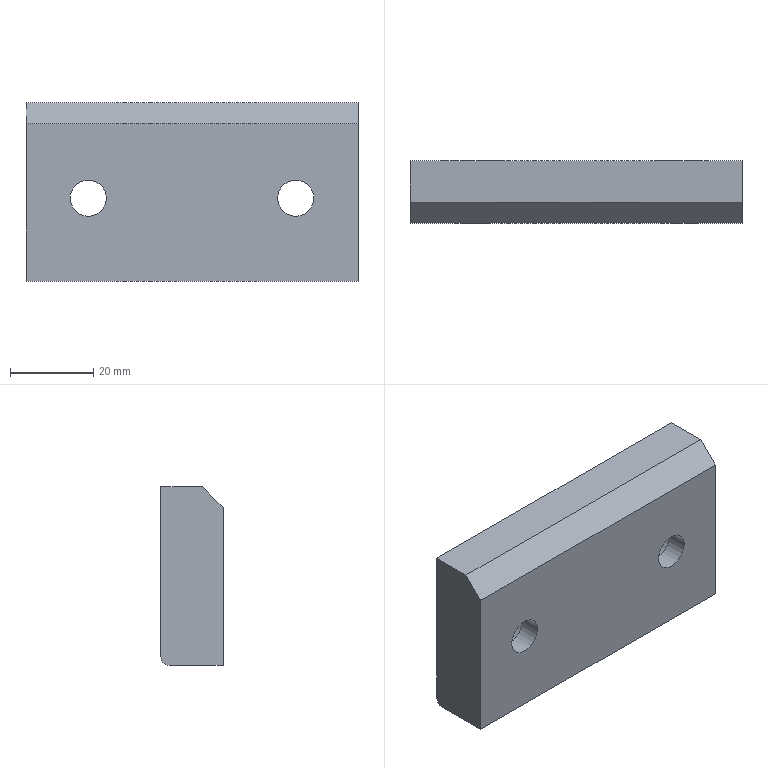Part | STEP file | 1_id1026_x_t | 1 solid | 14 faces | box 80 x 15 x 43 mm | volume 46403 mm3 | plane 9 | cylinder 5 | commonest cylinder face diameters 8.7 x2 15 x2 4 x1
STEP:
#1=CARTESIAN_POINT('',(0.,0.,0.));
#2=DIRECTION('',(0.,0.,1.));
#3=DIRECTION('',(1.,0.,0.));
#4=AXIS2_PLACEMENT_3D('',#1,#2,#3);
#5=CARTESIAN_POINT('',(787.926,422.974,-82.813));
#6=VERTEX_POINT('',#5);
#7=CARTESIAN_POINT('',(787.926,409.974,-82.813));
#8=VERTEX_POINT('',#7);
#9=CARTESIAN_POINT('',(787.926,422.974,-82.813));
#10=DIRECTION('',(0.,-1.,0.));
#11=VECTOR('',#10,1.);
#12=LINE('',#9,#11);
#13=CARTESIAN_POINT('',(787.926,409.974,-82.813));
#14=DIRECTION('',(1.,0.,0.));
#15=DIRECTION('',(0.,1.,0.));
#16=AXIS2_PLACEMENT_3D('',#13,#14,#15);
#17=PLANE('',#16);
#18=CARTESIAN_POINT('',(13.,0.));
#19=DIRECTION('',(-1.,0.));
#20=VECTOR('',#19,1.);
#21=LINE('',#18,#20);
#22=(GEOMETRIC_REPRESENTATION_CONTEXT(2)PARAMETRIC_REPRESENTATION_CONTEXT()REPRESENTATION_CONTEXT('',''));
#23=DEFINITIONAL_REPRESENTATION('',(#21),#22);
#24=PCURVE('',#17,#23);
#25=CARTESIAN_POINT('',(707.926,409.974,-82.813));
#26=DIRECTION('',(0.,0.,1.));
#27=DIRECTION('',(-1.,0.,0.));
#28=AXIS2_PLACEMENT_3D('',#25,#26,#27);
#29=PLANE('',#28);
#30=CARTESIAN_POINT('',(-80.,-13.));
#31=DIRECTION('',(0.,1.));
#32=VECTOR('',#31,1.);
#33=LINE('',#30,#32);
#34=(GEOMETRIC_REPRESENTATION_CONTEXT(2)PARAMETRIC_REPRESENTATION_CONTEXT()REPRESENTATION_CONTEXT('',''));
#35=DEFINITIONAL_REPRESENTATION('',(#33),#34);
#36=PCURVE('',#29,#35);
#37=SURFACE_CURVE('',#12,(#24,#36),.PCURVE_S1.);
#38=EDGE_CURVE('',#6,#8,#37,.T.);
#39=ORIENTED_EDGE('',*,*,#38,.F.);
#40=CARTESIAN_POINT('',(787.926,424.974,-80.813));
#41=VERTEX_POINT('',#40);
#42=CARTESIAN_POINT('',(787.926,422.974,-80.813));
#43=DIRECTION('',(1.,0.,0.));
#44=DIRECTION('',(0.,0.,-1.));
#45=AXIS2_PLACEMENT_3D('',#42,#43,#44);
#46=CIRCLE('',#45,2.);
#47=CARTESIAN_POINT('',(13.,2.));
#48=DIRECTION('',(0.,-1.));
#49=AXIS2_PLACEMENT_2D('',#47,#48);
#50=CIRCLE('',#49,2.);
#51=(GEOMETRIC_REPRESENTATION_CONTEXT(2)PARAMETRIC_REPRESENTATION_CONTEXT()REPRESENTATION_CONTEXT('',''));
#52=DEFINITIONAL_REPRESENTATION('',(#50),#51);
#53=PCURVE('',#17,#52);
#54=CARTESIAN_POINT('',(787.926,422.974,-80.813));
#55=DIRECTION('',(-1.,0.,0.));
#56=DIRECTION('',(0.,0.,1.));
#57=AXIS2_PLACEMENT_3D('',#54,#55,#56);
#58=CYLINDRICAL_SURFACE('',#57,2.);
#59=CARTESIAN_POINT('',(3.142,0.));
#60=DIRECTION('',(-1.,0.));
#61=VECTOR('',#60,1.);
#62=LINE('',#59,#61);
#63=(GEOMETRIC_REPRESENTATION_CONTEXT(2)PARAMETRIC_REPRESENTATION_CONTEXT()REPRESENTATION_CONTEXT('',''));
#64=DEFINITIONAL_REPRESENTATION('',(#62),#63);
#65=PCURVE('',#58,#64);
#66=SURFACE_CURVE('',#46,(#53,#65),.PCURVE_S1.);
#67=EDGE_CURVE('',#6,#41,#66,.T.);
#68=ORIENTED_EDGE('',*,*,#67,.T.);
#69=CARTESIAN_POINT('',(787.926,424.974,-39.813));
#70=VERTEX_POINT('',#69);
#71=CARTESIAN_POINT('',(787.926,424.974,-39.813));
#72=DIRECTION('',(0.,0.,-1.));
#73=VECTOR('',#72,1.);
#74=LINE('',#71,#73);
#75=CARTESIAN_POINT('',(15.,43.));
#76=DIRECTION('',(0.,-1.));
#77=VECTOR('',#76,1.);
#78=LINE('',#75,#77);
#79=(GEOMETRIC_REPRESENTATION_CONTEXT(2)PARAMETRIC_REPRESENTATION_CONTEXT()REPRESENTATION_CONTEXT('',''));
#80=DEFINITIONAL_REPRESENTATION('',(#78),#79);
#81=PCURVE('',#17,#80);
#82=CARTESIAN_POINT('',(787.926,424.974,-82.813));
#83=DIRECTION('',(0.,1.,0.));
#84=DIRECTION('',(0.,0.,1.));
#85=AXIS2_PLACEMENT_3D('',#82,#83,#84);
#86=PLANE('',#85);
#87=CARTESIAN_POINT('',(43.,0.));
#88=DIRECTION('',(-1.,0.));
#89=VECTOR('',#88,1.);
#90=LINE('',#87,#89);
#91=(GEOMETRIC_REPRESENTATION_CONTEXT(2)PARAMETRIC_REPRESENTATION_CONTEXT()REPRESENTATION_CONTEXT('',''));
#92=DEFINITIONAL_REPRESENTATION('',(#90),#91);
#93=PCURVE('',#86,#92);
#94=SURFACE_CURVE('',#74,(#81,#93),.PCURVE_S1.);
#95=EDGE_CURVE('',#70,#41,#94,.T.);
#96=ORIENTED_EDGE('',*,*,#95,.F.);
#97=CARTESIAN_POINT('',(787.926,414.974,-39.813));
#98=VERTEX_POINT('',#97);
#99=CARTESIAN_POINT('',(787.926,424.974,-39.813));
#100=DIRECTION('',(0.,-1.,0.));
#101=VECTOR('',#100,1.);
#102=LINE('',#99,#101);
#103=CARTESIAN_POINT('',(15.,43.));
#104=DIRECTION('',(-1.,0.));
#105=VECTOR('',#104,1.);
#106=LINE('',#103,#105);
#107=(GEOMETRIC_REPRESENTATION_CONTEXT(2)PARAMETRIC_REPRESENTATION_CONTEXT()REPRESENTATION_CONTEXT('',''));
#108=DEFINITIONAL_REPRESENTATION('',(#106),#107);
#109=PCURVE('',#17,#108);
#110=CARTESIAN_POINT('',(707.926,409.974,-39.813));
#111=DIRECTION('',(0.,0.,1.));
#112=DIRECTION('',(-1.,0.,0.));
#113=AXIS2_PLACEMENT_3D('',#110,#111,#112);
#114=PLANE('',#113);
#115=CARTESIAN_POINT('',(-80.,-15.));
#116=DIRECTION('',(0.,1.));
#117=VECTOR('',#116,1.);
#118=LINE('',#115,#117);
#119=(GEOMETRIC_REPRESENTATION_CONTEXT(2)PARAMETRIC_REPRESENTATION_CONTEXT()REPRESENTATION_CONTEXT('',''));
#120=DEFINITIONAL_REPRESENTATION('',(#118),#119);
#121=PCURVE('',#114,#120);
#122=SURFACE_CURVE('',#102,(#109,#121),.PCURVE_S1.);
#123=EDGE_CURVE('',#70,#98,#122,.T.);
#124=ORIENTED_EDGE('',*,*,#123,.T.);
#125=CARTESIAN_POINT('',(787.926,409.974,-44.813));
#126=VERTEX_POINT('',#125);
#127=CARTESIAN_POINT('',(787.926,414.974,-39.813));
#128=DIRECTION('',(0.,-0.7071,-0.7071));
#129=VECTOR('',#128,1.);
#130=LINE('',#127,#129);
#131=CARTESIAN_POINT('',(5.,43.));
#132=DIRECTION('',(-0.7071,-0.7071));
#133=VECTOR('',#132,1.);
#134=LINE('',#131,#133);
#135=(GEOMETRIC_REPRESENTATION_CONTEXT(2)PARAMETRIC_REPRESENTATION_CONTEXT()REPRESENTATION_CONTEXT('',''));
#136=DEFINITIONAL_REPRESENTATION('',(#134),#135);
#137=PCURVE('',#17,#136);
#138=CARTESIAN_POINT('',(707.926,409.974,-44.813));
#139=DIRECTION('',(0.,0.7071,-0.7071));
#140=DIRECTION('',(0.,-0.7071,-0.7071));
#141=AXIS2_PLACEMENT_3D('',#138,#139,#140);
#142=PLANE('',#141);
#143=CARTESIAN_POINT('',(-7.071,-80.));
#144=DIRECTION('',(1.,0.));
#145=VECTOR('',#144,1.);
#146=LINE('',#143,#145);
#147=(GEOMETRIC_REPRESENTATION_CONTEXT(2)PARAMETRIC_REPRESENTATION_CONTEXT()REPRESENTATION_CONTEXT('',''));
#148=DEFINITIONAL_REPRESENTATION('',(#146),#147);
#149=PCURVE('',#142,#148);
#150=SURFACE_CURVE('',#130,(#137,#149),.PCURVE_S1.);
#151=EDGE_CURVE('',#98,#126,#150,.T.);
#152=ORIENTED_EDGE('',*,*,#151,.T.);
#153=CARTESIAN_POINT('',(787.926,409.974,-44.813));
#154=DIRECTION('',(0.,0.,-1.));
#155=VECTOR('',#154,1.);
#156=LINE('',#153,#155);
#157=CARTESIAN_POINT('',(0.,38.));
#158=DIRECTION('',(0.,-1.));
#159=VECTOR('',#158,1.);
#160=LINE('',#157,#159);
#161=(GEOMETRIC_REPRESENTATION_CONTEXT(2)PARAMETRIC_REPRESENTATION_CONTEXT()REPRESENTATION_CONTEXT('',''));
#162=DEFINITIONAL_REPRESENTATION('',(#160),#161);
#163=PCURVE('',#17,#162);
#164=CARTESIAN_POINT('',(707.926,409.974,-82.813));
#165=DIRECTION('',(0.,-1.,0.));
#166=DIRECTION('',(-1.,0.,0.));
#167=AXIS2_PLACEMENT_3D('',#164,#165,#166);
#168=PLANE('',#167);
#169=CARTESIAN_POINT('',(-80.,-38.));
#170=DIRECTION('',(0.,1.));
#171=VECTOR('',#170,1.);
#172=LINE('',#169,#171);
#173=(GEOMETRIC_REPRESENTATION_CONTEXT(2)PARAMETRIC_REPRESENTATION_CONTEXT()REPRESENTATION_CONTEXT('',''));
#174=DEFINITIONAL_REPRESENTATION('',(#172),#173);
#175=PCURVE('',#168,#174);
#176=SURFACE_CURVE('',#156,(#163,#175),.PCURVE_S1.);
#177=EDGE_CURVE('',#126,#8,#176,.T.);
#178=ORIENTED_EDGE('',*,*,#177,.T.);
#179=EDGE_LOOP('',(#39,#68,#96,#124,#152,#178));
#180=FACE_BOUND('',#179,.T.);
#181=ADVANCED_FACE('',(#180),#17,.T.);
#182=CARTESIAN_POINT('',(707.926,409.974,-82.813));
#183=VERTEX_POINT('',#182);
#184=CARTESIAN_POINT('',(787.926,409.974,-82.813));
#185=DIRECTION('',(-1.,0.,0.));
#186=VECTOR('',#185,1.);
#187=LINE('',#184,#186);
#188=CARTESIAN_POINT('',(-80.,0.));
#189=DIRECTION('',(1.,0.));
#190=VECTOR('',#189,1.);
#191=LINE('',#188,#190);
#192=(GEOMETRIC_REPRESENTATION_CONTEXT(2)PARAMETRIC_REPRESENTATION_CONTEXT()REPRESENTATION_CONTEXT('',''));
#193=DEFINITIONAL_REPRESENTATION('',(#191),#192);
#194=PCURVE('',#168,#193);
#195=CARTESIAN_POINT('',(-80.,0.));
#196=DIRECTION('',(1.,0.));
#197=VECTOR('',#196,1.);
#198=LINE('',#195,#197);
#199=(GEOMETRIC_REPRESENTATION_CONTEXT(2)PARAMETRIC_REPRESENTATION_CONTEXT()REPRESENTATION_CONTEXT('',''));
#200=DEFINITIONAL_REPRESENTATION('',(#198),#199);
#201=PCURVE('',#29,#200);
#202=SURFACE_CURVE('',#187,(#194,#201),.PCURVE_S1.);
#203=EDGE_CURVE('',#8,#183,#202,.T.);
#204=ORIENTED_EDGE('',*,*,#203,.F.);
#205=ORIENTED_EDGE('',*,*,#177,.F.);
#206=CARTESIAN_POINT('',(707.926,409.974,-44.813));
#207=VERTEX_POINT('',#206);
#208=CARTESIAN_POINT('',(787.926,409.974,-44.813));
#209=DIRECTION('',(-1.,0.,0.));
#210=VECTOR('',#209,1.);
#211=LINE('',#208,#210);
#212=CARTESIAN_POINT('',(-80.,-38.));
#213=DIRECTION('',(1.,0.));
#214=VECTOR('',#213,1.);
#215=LINE('',#212,#214);
#216=(GEOMETRIC_REPRESENTATION_CONTEXT(2)PARAMETRIC_REPRESENTATION_CONTEXT()REPRESENTATION_CONTEXT('',''));
#217=DEFINITIONAL_REPRESENTATION('',(#215),#216);
#218=PCURVE('',#168,#217);
#219=CARTESIAN_POINT('',(0.,-80.));
#220=DIRECTION('',(0.,1.));
#221=VECTOR('',#220,1.);
#222=LINE('',#219,#221);
#223=(GEOMETRIC_REPRESENTATION_CONTEXT(2)PARAMETRIC_REPRESENTATION_CONTEXT()REPRESENTATION_CONTEXT('',''));
#224=DEFINITIONAL_REPRESENTATION('',(#222),#223);
#225=PCURVE('',#142,#224);
#226=SURFACE_CURVE('',#211,(#218,#225),.PCURVE_S1.);
#227=EDGE_CURVE('',#126,#207,#226,.T.);
#228=ORIENTED_EDGE('',*,*,#227,.T.);
#229=CARTESIAN_POINT('',(707.926,409.974,-44.813));
#230=DIRECTION('',(0.,0.,-1.));
#231=VECTOR('',#230,1.);
#232=LINE('',#229,#231);
#233=CARTESIAN_POINT('',(0.,-38.));
#234=DIRECTION('',(0.,1.));
#235=VECTOR('',#234,1.);
#236=LINE('',#233,#235);
#237=(GEOMETRIC_REPRESENTATION_CONTEXT(2)PARAMETRIC_REPRESENTATION_CONTEXT()REPRESENTATION_CONTEXT('',''));
#238=DEFINITIONAL_REPRESENTATION('',(#236),#237);
#239=PCURVE('',#168,#238);
#240=CARTESIAN_POINT('',(707.926,429.974,-82.813));
#241=DIRECTION('',(-1.,0.,0.));
#242=DIRECTION('',(0.,0.,-1.));
#243=AXIS2_PLACEMENT_3D('',#240,#241,#242);
#244=PLANE('',#243);
#245=CARTESIAN_POINT('',(-38.,20.));
#246=DIRECTION('',(1.,0.));
#247=VECTOR('',#246,1.);
#248=LINE('',#245,#247);
#249=(GEOMETRIC_REPRESENTATION_CONTEXT(2)PARAMETRIC_REPRESENTATION_CONTEXT()REPRESENTATION_CONTEXT('',''));
#250=DEFINITIONAL_REPRESENTATION('',(#248),#249);
#251=PCURVE('',#244,#250);
#252=SURFACE_CURVE('',#232,(#239,#251),.PCURVE_S1.);
#253=EDGE_CURVE('',#207,#183,#252,.T.);
#254=ORIENTED_EDGE('',*,*,#253,.T.);
#255=EDGE_LOOP('',(#204,#205,#228,#254));
#256=FACE_BOUND('',#255,.T.);
#257=CARTESIAN_POINT('',(772.926,409.974,-58.463));
#258=VERTEX_POINT('',#257);
#259=CARTESIAN_POINT('',(772.926,409.974,-62.813));
#260=DIRECTION('',(0.,1.,0.));
#261=DIRECTION('',(0.,0.,1.));
#262=AXIS2_PLACEMENT_3D('',#259,#260,#261);
#263=CIRCLE('',#262,4.35);
#264=CARTESIAN_POINT('',(-65.,-24.35));
#265=CARTESIAN_POINT('',(-72.534,-24.35));
#266=CARTESIAN_POINT('',(-68.767,-17.825));
#267=CARTESIAN_POINT('',(-65.,-11.3));
#268=CARTESIAN_POINT('',(-61.233,-17.825));
#269=CARTESIAN_POINT('',(-57.466,-24.35));
#270=CARTESIAN_POINT('',(-65.,-24.35));
#271=(BOUNDED_CURVE()B_SPLINE_CURVE(2,(#264,#265,#266,#267,#268,#269,#270),.UNSPECIFIED.,.T.,.F.)B_SPLINE_CURVE_WITH_KNOTS((1,2,2,2,2,1),(-2.094,0.,2.094,4.189,6.283,8.378),.UNSPECIFIED.)CURVE()GEOMETRIC_REPRESENTATION_ITEM()RATIONAL_B_SPLINE_CURVE((1.,0.5,1.,0.5,1.,0.5,1.))REPRESENTATION_ITEM(''));
#272=(GEOMETRIC_REPRESENTATION_CONTEXT(2)PARAMETRIC_REPRESENTATION_CONTEXT()REPRESENTATION_CONTEXT('',''));
#273=DEFINITIONAL_REPRESENTATION('',(#271),#272);
#274=PCURVE('',#168,#273);
#275=CARTESIAN_POINT('',(772.926,409.824,-62.813));
#276=DIRECTION('',(0.,-1.,0.));
#277=DIRECTION('',(0.,0.,-1.));
#278=AXIS2_PLACEMENT_3D('',#275,#276,#277);
#279=CYLINDRICAL_SURFACE('',#278,4.35);
#280=CARTESIAN_POINT('',(9.425,-0.15));
#281=DIRECTION('',(-1.,0.));
#282=VECTOR('',#281,1.);
#283=LINE('',#280,#282);
#284=(GEOMETRIC_REPRESENTATION_CONTEXT(2)PARAMETRIC_REPRESENTATION_CONTEXT()REPRESENTATION_CONTEXT('',''));
#285=DEFINITIONAL_REPRESENTATION('',(#283),#284);
#286=PCURVE('',#279,#285);
#287=SURFACE_CURVE('',#263,(#274,#286),.PCURVE_S1.);
#288=EDGE_CURVE('',#258,#258,#287,.T.);
#289=ORIENTED_EDGE('',*,*,#288,.T.);
#290=EDGE_LOOP('',(#289));
#291=FACE_BOUND('',#290,.T.);
#292=CARTESIAN_POINT('',(722.926,409.974,-58.463));
#293=VERTEX_POINT('',#292);
#294=CARTESIAN_POINT('',(722.926,409.974,-62.813));
#295=DIRECTION('',(0.,1.,0.));
#296=DIRECTION('',(0.,0.,1.));
#297=AXIS2_PLACEMENT_3D('',#294,#295,#296);
#298=CIRCLE('',#297,4.35);
#299=CARTESIAN_POINT('',(-15.,-24.35));
#300=CARTESIAN_POINT('',(-22.534,-24.35));
#301=CARTESIAN_POINT('',(-18.767,-17.825));
#302=CARTESIAN_POINT('',(-15.,-11.3));
#303=CARTESIAN_POINT('',(-11.233,-17.825));
#304=CARTESIAN_POINT('',(-7.466,-24.35));
#305=CARTESIAN_POINT('',(-15.,-24.35));
#306=(BOUNDED_CURVE()B_SPLINE_CURVE(2,(#299,#300,#301,#302,#303,#304,#305),.UNSPECIFIED.,.T.,.F.)B_SPLINE_CURVE_WITH_KNOTS((1,2,2,2,2,1),(-2.094,0.,2.094,4.189,6.283,8.378),.UNSPECIFIED.)CURVE()GEOMETRIC_REPRESENTATION_ITEM()RATIONAL_B_SPLINE_CURVE((1.,0.5,1.,0.5,1.,0.5,1.))REPRESENTATION_ITEM(''));
#307=(GEOMETRIC_REPRESENTATION_CONTEXT(2)PARAMETRIC_REPRESENTATION_CONTEXT()REPRESENTATION_CONTEXT('',''));
#308=DEFINITIONAL_REPRESENTATION('',(#306),#307);
#309=PCURVE('',#168,#308);
#310=CARTESIAN_POINT('',(722.926,409.824,-62.813));
#311=DIRECTION('',(0.,-1.,0.));
#312=DIRECTION('',(-1.,0.,0.));
#313=AXIS2_PLACEMENT_3D('',#310,#311,#312);
#314=CYLINDRICAL_SURFACE('',#313,4.35);
#315=CARTESIAN_POINT('',(10.996,-0.15));
#316=DIRECTION('',(-1.,0.));
#317=VECTOR('',#316,1.);
#318=LINE('',#315,#317);
#319=(GEOMETRIC_REPRESENTATION_CONTEXT(2)PARAMETRIC_REPRESENTATION_CONTEXT()REPRESENTATION_CONTEXT('',''));
#320=DEFINITIONAL_REPRESENTATION('',(#318),#319);
#321=PCURVE('',#314,#320);
#322=SURFACE_CURVE('',#298,(#309,#321),.PCURVE_S1.);
#323=EDGE_CURVE('',#293,#293,#322,.T.);
#324=ORIENTED_EDGE('',*,*,#323,.T.);
#325=EDGE_LOOP('',(#324));
#326=FACE_BOUND('',#325,.T.);
#327=ADVANCED_FACE('',(#256,#291,#326),#168,.T.);
#328=CARTESIAN_POINT('',(707.926,424.974,-39.813));
#329=VERTEX_POINT('',#328);
#330=CARTESIAN_POINT('',(707.926,424.974,-80.813));
#331=VERTEX_POINT('',#330);
#332=CARTESIAN_POINT('',(707.926,424.974,-39.813));
#333=DIRECTION('',(0.,0.,-1.));
#334=VECTOR('',#333,1.);
#335=LINE('',#332,#334);
#336=CARTESIAN_POINT('',(-43.,5.));
#337=DIRECTION('',(1.,0.));
#338=VECTOR('',#337,1.);
#339=LINE('',#336,#338);
#340=(GEOMETRIC_REPRESENTATION_CONTEXT(2)PARAMETRIC_REPRESENTATION_CONTEXT()REPRESENTATION_CONTEXT('',''));
#341=DEFINITIONAL_REPRESENTATION('',(#339),#340);
#342=PCURVE('',#244,#341);
#343=CARTESIAN_POINT('',(43.,-80.));
#344=DIRECTION('',(-1.,0.));
#345=VECTOR('',#344,1.);
#346=LINE('',#343,#345);
#347=(GEOMETRIC_REPRESENTATION_CONTEXT(2)PARAMETRIC_REPRESENTATION_CONTEXT()REPRESENTATION_CONTEXT('',''));
#348=DEFINITIONAL_REPRESENTATION('',(#346),#347);
#349=PCURVE('',#86,#348);
#350=SURFACE_CURVE('',#335,(#342,#349),.PCURVE_S1.);
#351=EDGE_CURVE('',#329,#331,#350,.T.);
#352=ORIENTED_EDGE('',*,*,#351,.T.);
#353=CARTESIAN_POINT('',(707.926,422.974,-82.813));
#354=VERTEX_POINT('',#353);
#355=CARTESIAN_POINT('',(707.926,422.974,-80.813));
#356=DIRECTION('',(-1.,0.,0.));
#357=DIRECTION('',(0.,1.,0.));
#358=AXIS2_PLACEMENT_3D('',#355,#356,#357);
#359=CIRCLE('',#358,2.);
#360=CARTESIAN_POINT('',(-2.,7.));
#361=DIRECTION('',(0.,-1.));
#362=AXIS2_PLACEMENT_2D('',#360,#361);
#363=CIRCLE('',#362,2.);
#364=(GEOMETRIC_REPRESENTATION_CONTEXT(2)PARAMETRIC_REPRESENTATION_CONTEXT()REPRESENTATION_CONTEXT('',''));
#365=DEFINITIONAL_REPRESENTATION('',(#363),#364);
#366=PCURVE('',#244,#365);
#367=CARTESIAN_POINT('',(1.571,80.));
#368=DIRECTION('',(1.,0.));
#369=VECTOR('',#368,1.);
#370=LINE('',#367,#369);
#371=(GEOMETRIC_REPRESENTATION_CONTEXT(2)PARAMETRIC_REPRESENTATION_CONTEXT()REPRESENTATION_CONTEXT('',''));
#372=DEFINITIONAL_REPRESENTATION('',(#370),#371);
#373=PCURVE('',#58,#372);
#374=SURFACE_CURVE('',#359,(#366,#373),.PCURVE_S1.);
#375=EDGE_CURVE('',#331,#354,#374,.T.);
#376=ORIENTED_EDGE('',*,*,#375,.T.);
#377=CARTESIAN_POINT('',(707.926,409.974,-82.813));
#378=DIRECTION('',(0.,1.,0.));
#379=VECTOR('',#378,1.);
#380=LINE('',#377,#379);
#381=CARTESIAN_POINT('',(0.,20.));
#382=DIRECTION('',(0.,-1.));
#383=VECTOR('',#382,1.);
#384=LINE('',#381,#383);
#385=(GEOMETRIC_REPRESENTATION_CONTEXT(2)PARAMETRIC_REPRESENTATION_CONTEXT()REPRESENTATION_CONTEXT('',''));
#386=DEFINITIONAL_REPRESENTATION('',(#384),#385);
#387=PCURVE('',#244,#386);
#388=CARTESIAN_POINT('',(0.,0.));
#389=DIRECTION('',(0.,-1.));
#390=VECTOR('',#389,1.);
#391=LINE('',#388,#390);
#392=(GEOMETRIC_REPRESENTATION_CONTEXT(2)PARAMETRIC_REPRESENTATION_CONTEXT()REPRESENTATION_CONTEXT('',''));
#393=DEFINITIONAL_REPRESENTATION('',(#391),#392);
#394=PCURVE('',#29,#393);
#395=SURFACE_CURVE('',#380,(#387,#394),.PCURVE_S1.);
#396=EDGE_CURVE('',#183,#354,#395,.T.);
#397=ORIENTED_EDGE('',*,*,#396,.F.);
#398=ORIENTED_EDGE('',*,*,#253,.F.);
#399=CARTESIAN_POINT('',(707.926,414.974,-39.813));
#400=VERTEX_POINT('',#399);
#401=CARTESIAN_POINT('',(707.926,409.974,-44.813));
#402=DIRECTION('',(0.,0.7071,0.7071));
#403=VECTOR('',#402,1.);
#404=LINE('',#401,#403);
#405=CARTESIAN_POINT('',(-38.,20.));
#406=DIRECTION('',(-0.7071,-0.7071));
#407=VECTOR('',#406,1.);
#408=LINE('',#405,#407);
#409=(GEOMETRIC_REPRESENTATION_CONTEXT(2)PARAMETRIC_REPRESENTATION_CONTEXT()REPRESENTATION_CONTEXT('',''));
#410=DEFINITIONAL_REPRESENTATION('',(#408),#409);
#411=PCURVE('',#244,#410);
#412=CARTESIAN_POINT('',(0.,0.));
#413=DIRECTION('',(-1.,0.));
#414=VECTOR('',#413,1.);
#415=LINE('',#412,#414);
#416=(GEOMETRIC_REPRESENTATION_CONTEXT(2)PARAMETRIC_REPRESENTATION_CONTEXT()REPRESENTATION_CONTEXT('',''));
#417=DEFINITIONAL_REPRESENTATION('',(#415),#416);
#418=PCURVE('',#142,#417);
#419=SURFACE_CURVE('',#404,(#411,#418),.PCURVE_S1.);
#420=EDGE_CURVE('',#207,#400,#419,.T.);
#421=ORIENTED_EDGE('',*,*,#420,.T.);
#422=CARTESIAN_POINT('',(707.926,414.974,-39.813));
#423=DIRECTION('',(0.,1.,0.));
#424=VECTOR('',#423,1.);
#425=LINE('',#422,#424);
#426=CARTESIAN_POINT('',(-43.,15.));
#427=DIRECTION('',(0.,-1.));
#428=VECTOR('',#427,1.);
#429=LINE('',#426,#428);
#430=(GEOMETRIC_REPRESENTATION_CONTEXT(2)PARAMETRIC_REPRESENTATION_CONTEXT()REPRESENTATION_CONTEXT('',''));
#431=DEFINITIONAL_REPRESENTATION('',(#429),#430);
#432=PCURVE('',#244,#431);
#433=CARTESIAN_POINT('',(0.,-5.));
#434=DIRECTION('',(0.,-1.));
#435=VECTOR('',#434,1.);
#436=LINE('',#433,#435);
#437=(GEOMETRIC_REPRESENTATION_CONTEXT(2)PARAMETRIC_REPRESENTATION_CONTEXT()REPRESENTATION_CONTEXT('',''));
#438=DEFINITIONAL_REPRESENTATION('',(#436),#437);
#439=PCURVE('',#114,#438);
#440=SURFACE_CURVE('',#425,(#432,#439),.PCURVE_S1.);
#441=EDGE_CURVE('',#400,#329,#440,.T.);
#442=ORIENTED_EDGE('',*,*,#441,.T.);
#443=EDGE_LOOP('',(#352,#376,#397,#398,#421,#442));
#444=FACE_BOUND('',#443,.T.);
#445=ADVANCED_FACE('',(#444),#244,.T.);
#446=CARTESIAN_POINT('',(707.926,424.974,-39.813));
#447=DIRECTION('',(1.,0.,0.));
#448=VECTOR('',#447,1.);
#449=LINE('',#446,#448);
#450=CARTESIAN_POINT('',(0.,-15.));
#451=DIRECTION('',(-1.,0.));
#452=VECTOR('',#451,1.);
#453=LINE('',#450,#452);
#454=(GEOMETRIC_REPRESENTATION_CONTEXT(2)PARAMETRIC_REPRESENTATION_CONTEXT()REPRESENTATION_CONTEXT('',''));
#455=DEFINITIONAL_REPRESENTATION('',(#453),#454);
#456=PCURVE('',#114,#455);
#457=CARTESIAN_POINT('',(43.,-80.));
#458=DIRECTION('',(0.,1.));
#459=VECTOR('',#458,1.);
#460=LINE('',#457,#459);
#461=(GEOMETRIC_REPRESENTATION_CONTEXT(2)PARAMETRIC_REPRESENTATION_CONTEXT()REPRESENTATION_CONTEXT('',''));
#462=DEFINITIONAL_REPRESENTATION('',(#460),#461);
#463=PCURVE('',#86,#462);
#464=SURFACE_CURVE('',#449,(#456,#463),.PCURVE_S1.);
#465=EDGE_CURVE('',#329,#70,#464,.T.);
#466=ORIENTED_EDGE('',*,*,#465,.F.);
#467=ORIENTED_EDGE('',*,*,#441,.F.);
#468=CARTESIAN_POINT('',(707.926,414.974,-39.813));
#469=DIRECTION('',(1.,0.,0.));
#470=VECTOR('',#469,1.);
#471=LINE('',#468,#470);
#472=CARTESIAN_POINT('',(0.,-5.));
#473=DIRECTION('',(-1.,0.));
#474=VECTOR('',#473,1.);
#475=LINE('',#472,#474);
#476=(GEOMETRIC_REPRESENTATION_CONTEXT(2)PARAMETRIC_REPRESENTATION_CONTEXT()REPRESENTATION_CONTEXT('',''));
#477=DEFINITIONAL_REPRESENTATION('',(#475),#476);
#478=PCURVE('',#114,#477);
#479=CARTESIAN_POINT('',(-7.071,0.));
#480=DIRECTION('',(0.,-1.));
#481=VECTOR('',#480,1.);
#482=LINE('',#479,#481);
#483=(GEOMETRIC_REPRESENTATION_CONTEXT(2)PARAMETRIC_REPRESENTATION_CONTEXT()REPRESENTATION_CONTEXT('',''));
#484=DEFINITIONAL_REPRESENTATION('',(#482),#483);
#485=PCURVE('',#142,#484);
#486=SURFACE_CURVE('',#471,(#478,#485),.PCURVE_S1.);
#487=EDGE_CURVE('',#400,#98,#486,.T.);
#488=ORIENTED_EDGE('',*,*,#487,.T.);
#489=ORIENTED_EDGE('',*,*,#123,.F.);
#490=EDGE_LOOP('',(#466,#467,#488,#489));
#491=FACE_BOUND('',#490,.T.);
#492=ADVANCED_FACE('',(#491),#114,.T.);
#493=ORIENTED_EDGE('',*,*,#227,.F.);
#494=ORIENTED_EDGE('',*,*,#151,.F.);
#495=ORIENTED_EDGE('',*,*,#487,.F.);
#496=ORIENTED_EDGE('',*,*,#420,.F.);
#497=EDGE_LOOP('',(#493,#494,#495,#496));
#498=FACE_BOUND('',#497,.T.);
#499=ADVANCED_FACE('',(#498),#142,.F.);
#500=CARTESIAN_POINT('',(707.926,424.974,-80.813));
#501=DIRECTION('',(1.,0.,0.));
#502=VECTOR('',#501,1.);
#503=LINE('',#500,#502);
#504=CARTESIAN_POINT('',(2.,-80.));
#505=DIRECTION('',(0.,1.));
#506=VECTOR('',#505,1.);
#507=LINE('',#504,#506);
#508=(GEOMETRIC_REPRESENTATION_CONTEXT(2)PARAMETRIC_REPRESENTATION_CONTEXT()REPRESENTATION_CONTEXT('',''));
#509=DEFINITIONAL_REPRESENTATION('',(#507),#508);
#510=PCURVE('',#86,#509);
#511=CARTESIAN_POINT('',(1.571,80.));
#512=DIRECTION('',(0.,-1.));
#513=VECTOR('',#512,1.);
#514=LINE('',#511,#513);
#515=(GEOMETRIC_REPRESENTATION_CONTEXT(2)PARAMETRIC_REPRESENTATION_CONTEXT()REPRESENTATION_CONTEXT('',''));
#516=DEFINITIONAL_REPRESENTATION('',(#514),#515);
#517=PCURVE('',#58,#516);
#518=SURFACE_CURVE('',#503,(#510,#517),.PCURVE_S1.);
#519=EDGE_CURVE('',#331,#41,#518,.T.);
#520=ORIENTED_EDGE('',*,*,#519,.F.);
#521=ORIENTED_EDGE('',*,*,#351,.F.);
#522=ORIENTED_EDGE('',*,*,#465,.T.);
#523=ORIENTED_EDGE('',*,*,#95,.T.);
#524=EDGE_LOOP('',(#520,#521,#522,#523));
#525=FACE_BOUND('',#524,.T.);
#526=CARTESIAN_POINT('',(730.426,424.974,-62.813));
#527=VERTEX_POINT('',#526);
#528=CARTESIAN_POINT('',(715.426,424.974,-62.813));
#529=VERTEX_POINT('',#528);
#530=CARTESIAN_POINT('',(722.926,424.974,-62.813));
#531=DIRECTION('',(0.,-1.,0.));
#532=DIRECTION('',(1.,0.,0.));
#533=AXIS2_PLACEMENT_3D('',#530,#531,#532);
#534=CIRCLE('',#533,7.5);
#535=CARTESIAN_POINT('',(20.,-57.5));
#536=CARTESIAN_POINT('',(32.99,-57.5));
#537=CARTESIAN_POINT('',(26.495,-68.75));
#538=CARTESIAN_POINT('',(20.,-80.));
#539=CARTESIAN_POINT('',(13.505,-68.75));
#540=CARTESIAN_POINT('',(7.01,-57.5));
#541=CARTESIAN_POINT('',(20.,-57.5));
#542=(BOUNDED_CURVE()B_SPLINE_CURVE(2,(#535,#536,#537,#538,#539,#540,#541),.UNSPECIFIED.,.T.,.F.)B_SPLINE_CURVE_WITH_KNOTS((1,2,2,2,2,1),(-2.094,0.,2.094,4.189,6.283,8.378),.UNSPECIFIED.)CURVE()GEOMETRIC_REPRESENTATION_ITEM()RATIONAL_B_SPLINE_CURVE((1.,0.5,1.,0.5,1.,0.5,1.))REPRESENTATION_ITEM(''));
#543=(GEOMETRIC_REPRESENTATION_CONTEXT(2)PARAMETRIC_REPRESENTATION_CONTEXT()REPRESENTATION_CONTEXT('',''));
#544=DEFINITIONAL_REPRESENTATION('',(#542),#543);
#545=PCURVE('',#86,#544);
#546=CARTESIAN_POINT('',(722.926,414.974,-62.813));
#547=DIRECTION('',(0.,-1.,0.));
#548=DIRECTION('',(-1.,0.,0.));
#549=AXIS2_PLACEMENT_3D('',#546,#547,#548);
#550=CYLINDRICAL_SURFACE('',#549,7.5);
#551=CARTESIAN_POINT('',(3.142,-10.));
#552=DIRECTION('',(1.,0.));
#553=VECTOR('',#552,1.);
#554=LINE('',#551,#553);
#555=(GEOMETRIC_REPRESENTATION_CONTEXT(2)PARAMETRIC_REPRESENTATION_CONTEXT()REPRESENTATION_CONTEXT('',''));
#556=DEFINITIONAL_REPRESENTATION('',(#554),#555);
#557=PCURVE('',#550,#556);
#558=SURFACE_CURVE('',#534,(#545,#557),.PCURVE_S1.);
#559=EDGE_CURVE('',#527,#529,#558,.T.);
#560=ORIENTED_EDGE('',*,*,#559,.T.);
#561=CARTESIAN_POINT('',(722.926,424.974,-62.813));
#562=DIRECTION('',(0.,-1.,0.));
#563=DIRECTION('',(1.,0.,0.));
#564=AXIS2_PLACEMENT_3D('',#561,#562,#563);
#565=CIRCLE('',#564,7.5);
#566=CARTESIAN_POINT('',(20.,-57.5));
#567=CARTESIAN_POINT('',(32.99,-57.5));
#568=CARTESIAN_POINT('',(26.495,-68.75));
#569=CARTESIAN_POINT('',(20.,-80.));
#570=CARTESIAN_POINT('',(13.505,-68.75));
#571=CARTESIAN_POINT('',(7.01,-57.5));
#572=CARTESIAN_POINT('',(20.,-57.5));
#573=(BOUNDED_CURVE()B_SPLINE_CURVE(2,(#566,#567,#568,#569,#570,#571,#572),.UNSPECIFIED.,.T.,.F.)B_SPLINE_CURVE_WITH_KNOTS((1,2,2,2,2,1),(-2.094,0.,2.094,4.189,6.283,8.378),.UNSPECIFIED.)CURVE()GEOMETRIC_REPRESENTATION_ITEM()RATIONAL_B_SPLINE_CURVE((1.,0.5,1.,0.5,1.,0.5,1.))REPRESENTATION_ITEM(''));
#574=(GEOMETRIC_REPRESENTATION_CONTEXT(2)PARAMETRIC_REPRESENTATION_CONTEXT()REPRESENTATION_CONTEXT('',''));
#575=DEFINITIONAL_REPRESENTATION('',(#573),#574);
#576=PCURVE('',#86,#575);
#577=CARTESIAN_POINT('',(-3.142,-10.));
#578=DIRECTION('',(1.,0.));
#579=VECTOR('',#578,1.);
#580=LINE('',#577,#579);
#581=(GEOMETRIC_REPRESENTATION_CONTEXT(2)PARAMETRIC_REPRESENTATION_CONTEXT()REPRESENTATION_CONTEXT('',''));
#582=DEFINITIONAL_REPRESENTATION('',(#580),#581);
#583=PCURVE('',#550,#582);
#584=SURFACE_CURVE('',#565,(#576,#583),.PCURVE_S1.);
#585=EDGE_CURVE('',#529,#527,#584,.T.);
#586=ORIENTED_EDGE('',*,*,#585,.T.);
#587=EDGE_LOOP('',(#560,#586));
#588=FACE_BOUND('',#587,.T.);
#589=CARTESIAN_POINT('',(772.926,424.974,-55.313));
#590=VERTEX_POINT('',#589);
#591=CARTESIAN_POINT('',(772.926,424.974,-70.313));
#592=VERTEX_POINT('',#591);
#593=CARTESIAN_POINT('',(772.926,424.974,-62.813));
#594=DIRECTION('',(0.,-1.,0.));
#595=DIRECTION('',(0.,0.,1.));
#596=AXIS2_PLACEMENT_3D('',#593,#594,#595);
#597=CIRCLE('',#596,7.5);
#598=CARTESIAN_POINT('',(27.5,-15.));
#599=CARTESIAN_POINT('',(27.5,-27.99));
#600=CARTESIAN_POINT('',(16.25,-21.495));
#601=CARTESIAN_POINT('',(5.,-15.));
#602=CARTESIAN_POINT('',(16.25,-8.505));
#603=CARTESIAN_POINT('',(27.5,-2.01));
#604=CARTESIAN_POINT('',(27.5,-15.));
#605=(BOUNDED_CURVE()B_SPLINE_CURVE(2,(#598,#599,#600,#601,#602,#603,#604),.UNSPECIFIED.,.T.,.F.)B_SPLINE_CURVE_WITH_KNOTS((1,2,2,2,2,1),(-2.094,0.,2.094,4.189,6.283,8.378),.UNSPECIFIED.)CURVE()GEOMETRIC_REPRESENTATION_ITEM()RATIONAL_B_SPLINE_CURVE((1.,0.5,1.,0.5,1.,0.5,1.))REPRESENTATION_ITEM(''));
#606=(GEOMETRIC_REPRESENTATION_CONTEXT(2)PARAMETRIC_REPRESENTATION_CONTEXT()REPRESENTATION_CONTEXT('',''));
#607=DEFINITIONAL_REPRESENTATION('',(#605),#606);
#608=PCURVE('',#86,#607);
#609=CARTESIAN_POINT('',(772.926,414.974,-62.813));
#610=DIRECTION('',(0.,-1.,0.));
#611=DIRECTION('',(0.,0.,-1.));
#612=AXIS2_PLACEMENT_3D('',#609,#610,#611);
#613=CYLINDRICAL_SURFACE('',#612,7.5);
#614=CARTESIAN_POINT('',(3.142,-10.));
#615=DIRECTION('',(1.,0.));
#616=VECTOR('',#615,1.);
#617=LINE('',#614,#616);
#618=(GEOMETRIC_REPRESENTATION_CONTEXT(2)PARAMETRIC_REPRESENTATION_CONTEXT()REPRESENTATION_CONTEXT('',''));
#619=DEFINITIONAL_REPRESENTATION('',(#617),#618);
#620=PCURVE('',#613,#619);
#621=SURFACE_CURVE('',#597,(#608,#620),.PCURVE_S1.);
#622=EDGE_CURVE('',#590,#592,#621,.T.);
#623=ORIENTED_EDGE('',*,*,#622,.T.);
#624=CARTESIAN_POINT('',(772.926,424.974,-62.813));
#625=DIRECTION('',(0.,-1.,0.));
#626=DIRECTION('',(0.,0.,1.));
#627=AXIS2_PLACEMENT_3D('',#624,#625,#626);
#628=CIRCLE('',#627,7.5);
#629=CARTESIAN_POINT('',(27.5,-15.));
#630=CARTESIAN_POINT('',(27.5,-27.99));
#631=CARTESIAN_POINT('',(16.25,-21.495));
#632=CARTESIAN_POINT('',(5.,-15.));
#633=CARTESIAN_POINT('',(16.25,-8.505));
#634=CARTESIAN_POINT('',(27.5,-2.01));
#635=CARTESIAN_POINT('',(27.5,-15.));
#636=(BOUNDED_CURVE()B_SPLINE_CURVE(2,(#629,#630,#631,#632,#633,#634,#635),.UNSPECIFIED.,.T.,.F.)B_SPLINE_CURVE_WITH_KNOTS((1,2,2,2,2,1),(-2.094,0.,2.094,4.189,6.283,8.378),.UNSPECIFIED.)CURVE()GEOMETRIC_REPRESENTATION_ITEM()RATIONAL_B_SPLINE_CURVE((1.,0.5,1.,0.5,1.,0.5,1.))REPRESENTATION_ITEM(''));
#637=(GEOMETRIC_REPRESENTATION_CONTEXT(2)PARAMETRIC_REPRESENTATION_CONTEXT()REPRESENTATION_CONTEXT('',''));
#638=DEFINITIONAL_REPRESENTATION('',(#636),#637);
#639=PCURVE('',#86,#638);
#640=CARTESIAN_POINT('',(-3.142,-10.));
#641=DIRECTION('',(1.,0.));
#642=VECTOR('',#641,1.);
#643=LINE('',#640,#642);
#644=(GEOMETRIC_REPRESENTATION_CONTEXT(2)PARAMETRIC_REPRESENTATION_CONTEXT()REPRESENTATION_CONTEXT('',''));
#645=DEFINITIONAL_REPRESENTATION('',(#643),#644);
#646=PCURVE('',#613,#645);
#647=SURFACE_CURVE('',#628,(#639,#646),.PCURVE_S1.);
#648=EDGE_CURVE('',#592,#590,#647,.T.);
#649=ORIENTED_EDGE('',*,*,#648,.T.);
#650=EDGE_LOOP('',(#623,#649));
#651=FACE_BOUND('',#650,.T.);
#652=ADVANCED_FACE('',(#525,#588,#651),#86,.T.);
#653=CARTESIAN_POINT('',(787.926,422.974,-82.813));
#654=DIRECTION('',(-1.,0.,0.));
#655=VECTOR('',#654,1.);
#656=LINE('',#653,#655);
#657=CARTESIAN_POINT('',(3.142,0.));
#658=DIRECTION('',(0.,1.));
#659=VECTOR('',#658,1.);
#660=LINE('',#657,#659);
#661=(GEOMETRIC_REPRESENTATION_CONTEXT(2)PARAMETRIC_REPRESENTATION_CONTEXT()REPRESENTATION_CONTEXT('',''));
#662=DEFINITIONAL_REPRESENTATION('',(#660),#661);
#663=PCURVE('',#58,#662);
#664=CARTESIAN_POINT('',(-80.,-13.));
#665=DIRECTION('',(1.,0.));
#666=VECTOR('',#665,1.);
#667=LINE('',#664,#666);
#668=(GEOMETRIC_REPRESENTATION_CONTEXT(2)PARAMETRIC_REPRESENTATION_CONTEXT()REPRESENTATION_CONTEXT('',''));
#669=DEFINITIONAL_REPRESENTATION('',(#667),#668);
#670=PCURVE('',#29,#669);
#671=SURFACE_CURVE('',#656,(#663,#670),.PCURVE_S1.);
#672=EDGE_CURVE('',#6,#354,#671,.T.);
#673=ORIENTED_EDGE('',*,*,#672,.T.);
#674=ORIENTED_EDGE('',*,*,#375,.F.);
#675=ORIENTED_EDGE('',*,*,#519,.T.);
#676=ORIENTED_EDGE('',*,*,#67,.F.);
#677=EDGE_LOOP('',(#673,#674,#675,#676));
#678=FACE_BOUND('',#677,.T.);
#679=ADVANCED_FACE('',(#678),#58,.T.);
#680=ORIENTED_EDGE('',*,*,#672,.F.);
#681=ORIENTED_EDGE('',*,*,#38,.T.);
#682=ORIENTED_EDGE('',*,*,#203,.T.);
#683=ORIENTED_EDGE('',*,*,#396,.T.);
#684=EDGE_LOOP('',(#680,#681,#682,#683));
#685=FACE_BOUND('',#684,.T.);
#686=ADVANCED_FACE('',(#685),#29,.F.);
#687=CARTESIAN_POINT('',(715.426,414.974,-62.813));
#688=VERTEX_POINT('',#687);
#689=CARTESIAN_POINT('',(722.926,414.974,-62.813));
#690=DIRECTION('',(0.,1.,0.));
#691=DIRECTION('',(-1.,0.,0.));
#692=AXIS2_PLACEMENT_3D('',#689,#690,#691);
#693=CIRCLE('',#692,7.5);
#694=CARTESIAN_POINT('',(6.283,0.));
#695=DIRECTION('',(-1.,0.));
#696=VECTOR('',#695,1.);
#697=LINE('',#694,#696);
#698=(GEOMETRIC_REPRESENTATION_CONTEXT(2)PARAMETRIC_REPRESENTATION_CONTEXT()REPRESENTATION_CONTEXT('',''));
#699=DEFINITIONAL_REPRESENTATION('',(#697),#698);
#700=PCURVE('',#550,#699);
#701=CARTESIAN_POINT('',(722.926,414.974,-62.813));
#702=DIRECTION('',(0.,-1.,0.));
#703=DIRECTION('',(-1.,0.,0.));
#704=AXIS2_PLACEMENT_3D('',#701,#702,#703);
#705=PLANE('',#704);
#706=CARTESIAN_POINT('',(7.5,0.));
#707=CARTESIAN_POINT('',(7.5,-12.99));
#708=CARTESIAN_POINT('',(-3.75,-6.495));
#709=CARTESIAN_POINT('',(-15.,0.));
#710=CARTESIAN_POINT('',(-3.75,6.495));
#711=CARTESIAN_POINT('',(7.5,12.99));
#712=CARTESIAN_POINT('',(7.5,0.));
#713=(BOUNDED_CURVE()B_SPLINE_CURVE(2,(#706,#707,#708,#709,#710,#711,#712),.UNSPECIFIED.,.T.,.F.)B_SPLINE_CURVE_WITH_KNOTS((1,2,2,2,2,1),(-2.094,0.,2.094,4.189,6.283,8.378),.UNSPECIFIED.)CURVE()GEOMETRIC_REPRESENTATION_ITEM()RATIONAL_B_SPLINE_CURVE((1.,0.5,1.,0.5,1.,0.5,1.))REPRESENTATION_ITEM(''));
#714=(GEOMETRIC_REPRESENTATION_CONTEXT(2)PARAMETRIC_REPRESENTATION_CONTEXT()REPRESENTATION_CONTEXT('',''));
#715=DEFINITIONAL_REPRESENTATION('',(#713),#714);
#716=PCURVE('',#705,#715);
#717=SURFACE_CURVE('',#693,(#700,#716),.PCURVE_S1.);
#718=EDGE_CURVE('',#688,#688,#717,.T.);
#719=ORIENTED_EDGE('',*,*,#718,.T.);
#720=CARTESIAN_POINT('',(715.426,424.974,-62.813));
#721=CARTESIAN_POINT('',(715.426,414.974,-62.813));
#722=B_SPLINE_CURVE_WITH_KNOTS('',1,(#720,#721),.UNSPECIFIED.,.F.,.F.,(2,2),(-10.,0.),.PIECEWISE_BEZIER_KNOTS.);
#723=CARTESIAN_POINT('',(0.,0.));
#724=DIRECTION('',(0.,1.));
#725=VECTOR('',#724,1.);
#726=LINE('',#723,#725);
#727=(GEOMETRIC_REPRESENTATION_CONTEXT(2)PARAMETRIC_REPRESENTATION_CONTEXT()REPRESENTATION_CONTEXT('',''));
#728=DEFINITIONAL_REPRESENTATION('',(#726),#727);
#729=PCURVE('',#550,#728);
#730=CARTESIAN_POINT('',(6.283,0.));
#731=DIRECTION('',(0.,1.));
#732=VECTOR('',#731,1.);
#733=LINE('',#730,#732);
#734=(GEOMETRIC_REPRESENTATION_CONTEXT(2)PARAMETRIC_REPRESENTATION_CONTEXT()REPRESENTATION_CONTEXT('',''));
#735=DEFINITIONAL_REPRESENTATION('',(#733),#734);
#736=PCURVE('',#550,#735);
#737=SEAM_CURVE('',#722,(#729,#736),.PCURVE_S1.);
#738=EDGE_CURVE('',#529,#688,#737,.T.);
#739=ORIENTED_EDGE('',*,*,#738,.F.);
#740=ORIENTED_EDGE('',*,*,#585,.T.);
#741=ORIENTED_EDGE('',*,*,#559,.T.);
#742=ORIENTED_EDGE('',*,*,#738,.T.);
#743=EDGE_LOOP('',(#719,#739,#740,#741,#742));
#744=FACE_BOUND('',#743,.F.);
#745=ADVANCED_FACE('',(#744),#550,.F.);
#746=ORIENTED_EDGE('',*,*,#718,.T.);
#747=EDGE_LOOP('',(#746));
#748=FACE_BOUND('',#747,.T.);
#749=CARTESIAN_POINT('',(722.926,414.974,-58.463));
#750=VERTEX_POINT('',#749);
#751=CARTESIAN_POINT('',(722.926,414.974,-62.813));
#752=DIRECTION('',(0.,-1.,0.));
#753=DIRECTION('',(0.,0.,1.));
#754=AXIS2_PLACEMENT_3D('',#751,#752,#753);
#755=CIRCLE('',#754,4.35);
#756=CARTESIAN_POINT('',(0.,0.));
#757=DIRECTION('',(0.,-1.));
#758=AXIS2_PLACEMENT_2D('',#756,#757);
#759=CIRCLE('',#758,4.35);
#760=(GEOMETRIC_REPRESENTATION_CONTEXT(2)PARAMETRIC_REPRESENTATION_CONTEXT()REPRESENTATION_CONTEXT('',''));
#761=DEFINITIONAL_REPRESENTATION('',(#759),#760);
#762=PCURVE('',#705,#761);
#763=CARTESIAN_POINT('',(4.712,-5.15));
#764=DIRECTION('',(1.,0.));
#765=VECTOR('',#764,1.);
#766=LINE('',#763,#765);
#767=(GEOMETRIC_REPRESENTATION_CONTEXT(2)PARAMETRIC_REPRESENTATION_CONTEXT()REPRESENTATION_CONTEXT('',''));
#768=DEFINITIONAL_REPRESENTATION('',(#766),#767);
#769=PCURVE('',#314,#768);
#770=SURFACE_CURVE('',#755,(#762,#769),.PCURVE_S1.);
#771=EDGE_CURVE('',#750,#750,#770,.T.);
#772=ORIENTED_EDGE('',*,*,#771,.T.);
#773=EDGE_LOOP('',(#772));
#774=FACE_BOUND('',#773,.T.);
#775=ADVANCED_FACE('',(#748,#774),#705,.F.);
#776=ORIENTED_EDGE('',*,*,#323,.T.);
#777=CARTESIAN_POINT('',(722.926,414.974,-58.463));
#778=CARTESIAN_POINT('',(722.926,409.974,-58.463));
#779=B_SPLINE_CURVE_WITH_KNOTS('',1,(#777,#778),.UNSPECIFIED.,.F.,.F.,(2,2),(-5.15,-0.15),.PIECEWISE_BEZIER_KNOTS.);
#780=CARTESIAN_POINT('',(4.712,0.));
#781=DIRECTION('',(0.,1.));
#782=VECTOR('',#781,1.);
#783=LINE('',#780,#782);
#784=(GEOMETRIC_REPRESENTATION_CONTEXT(2)PARAMETRIC_REPRESENTATION_CONTEXT()REPRESENTATION_CONTEXT('',''));
#785=DEFINITIONAL_REPRESENTATION('',(#783),#784);
#786=PCURVE('',#314,#785);
#787=CARTESIAN_POINT('',(10.996,0.));
#788=DIRECTION('',(0.,1.));
#789=VECTOR('',#788,1.);
#790=LINE('',#787,#789);
#791=(GEOMETRIC_REPRESENTATION_CONTEXT(2)PARAMETRIC_REPRESENTATION_CONTEXT()REPRESENTATION_CONTEXT('',''));
#792=DEFINITIONAL_REPRESENTATION('',(#790),#791);
#793=PCURVE('',#314,#792);
#794=SEAM_CURVE('',#779,(#786,#793),.PCURVE_S1.);
#795=EDGE_CURVE('',#750,#293,#794,.T.);
#796=ORIENTED_EDGE('',*,*,#795,.F.);
#797=ORIENTED_EDGE('',*,*,#771,.T.);
#798=ORIENTED_EDGE('',*,*,#795,.T.);
#799=EDGE_LOOP('',(#776,#796,#797,#798));
#800=FACE_BOUND('',#799,.F.);
#801=ADVANCED_FACE('',(#800),#314,.F.);
#802=CARTESIAN_POINT('',(772.926,414.974,-70.313));
#803=VERTEX_POINT('',#802);
#804=CARTESIAN_POINT('',(772.926,414.974,-62.813));
#805=DIRECTION('',(0.,1.,0.));
#806=DIRECTION('',(0.,0.,-1.));
#807=AXIS2_PLACEMENT_3D('',#804,#805,#806);
#808=CIRCLE('',#807,7.5);
#809=CARTESIAN_POINT('',(6.283,0.));
#810=DIRECTION('',(-1.,0.));
#811=VECTOR('',#810,1.);
#812=LINE('',#809,#811);
#813=(GEOMETRIC_REPRESENTATION_CONTEXT(2)PARAMETRIC_REPRESENTATION_CONTEXT()REPRESENTATION_CONTEXT('',''));
#814=DEFINITIONAL_REPRESENTATION('',(#812),#813);
#815=PCURVE('',#613,#814);
#816=CARTESIAN_POINT('',(772.926,414.974,-62.813));
#817=DIRECTION('',(0.,-1.,0.));
#818=DIRECTION('',(-1.,0.,0.));
#819=AXIS2_PLACEMENT_3D('',#816,#817,#818);
#820=PLANE('',#819);
#821=CARTESIAN_POINT('',(0.,7.5));
#822=CARTESIAN_POINT('',(12.99,7.5));
#823=CARTESIAN_POINT('',(6.495,-3.75));
#824=CARTESIAN_POINT('',(0.,-15.));
#825=CARTESIAN_POINT('',(-6.495,-3.75));
#826=CARTESIAN_POINT('',(-12.99,7.5));
#827=CARTESIAN_POINT('',(0.,7.5));
#828=(BOUNDED_CURVE()B_SPLINE_CURVE(2,(#821,#822,#823,#824,#825,#826,#827),.UNSPECIFIED.,.T.,.F.)B_SPLINE_CURVE_WITH_KNOTS((1,2,2,2,2,1),(-2.094,0.,2.094,4.189,6.283,8.378),.UNSPECIFIED.)CURVE()GEOMETRIC_REPRESENTATION_ITEM()RATIONAL_B_SPLINE_CURVE((1.,0.5,1.,0.5,1.,0.5,1.))REPRESENTATION_ITEM(''));
#829=(GEOMETRIC_REPRESENTATION_CONTEXT(2)PARAMETRIC_REPRESENTATION_CONTEXT()REPRESENTATION_CONTEXT('',''));
#830=DEFINITIONAL_REPRESENTATION('',(#828),#829);
#831=PCURVE('',#820,#830);
#832=SURFACE_CURVE('',#808,(#815,#831),.PCURVE_S1.);
#833=EDGE_CURVE('',#803,#803,#832,.T.);
#834=ORIENTED_EDGE('',*,*,#833,.T.);
#835=CARTESIAN_POINT('',(772.926,424.974,-70.313));
#836=CARTESIAN_POINT('',(772.926,414.974,-70.313));
#837=B_SPLINE_CURVE_WITH_KNOTS('',1,(#835,#836),.UNSPECIFIED.,.F.,.F.,(2,2),(-10.,0.),.PIECEWISE_BEZIER_KNOTS.);
#838=CARTESIAN_POINT('',(0.,0.));
#839=DIRECTION('',(0.,1.));
#840=VECTOR('',#839,1.);
#841=LINE('',#838,#840);
#842=(GEOMETRIC_REPRESENTATION_CONTEXT(2)PARAMETRIC_REPRESENTATION_CONTEXT()REPRESENTATION_CONTEXT('',''));
#843=DEFINITIONAL_REPRESENTATION('',(#841),#842);
#844=PCURVE('',#613,#843);
#845=CARTESIAN_POINT('',(6.283,0.));
#846=DIRECTION('',(0.,1.));
#847=VECTOR('',#846,1.);
#848=LINE('',#845,#847);
#849=(GEOMETRIC_REPRESENTATION_CONTEXT(2)PARAMETRIC_REPRESENTATION_CONTEXT()REPRESENTATION_CONTEXT('',''));
#850=DEFINITIONAL_REPRESENTATION('',(#848),#849);
#851=PCURVE('',#613,#850);
#852=SEAM_CURVE('',#837,(#844,#851),.PCURVE_S1.);
#853=EDGE_CURVE('',#592,#803,#852,.T.);
#854=ORIENTED_EDGE('',*,*,#853,.F.);
#855=ORIENTED_EDGE('',*,*,#648,.T.);
#856=ORIENTED_EDGE('',*,*,#622,.T.);
#857=ORIENTED_EDGE('',*,*,#853,.T.);
#858=EDGE_LOOP('',(#834,#854,#855,#856,#857));
#859=FACE_BOUND('',#858,.F.);
#860=ADVANCED_FACE('',(#859),#613,.F.);
#861=ORIENTED_EDGE('',*,*,#833,.T.);
#862=EDGE_LOOP('',(#861));
#863=FACE_BOUND('',#862,.T.);
#864=CARTESIAN_POINT('',(772.926,414.974,-58.463));
#865=VERTEX_POINT('',#864);
#866=CARTESIAN_POINT('',(772.926,414.974,-62.813));
#867=DIRECTION('',(0.,-1.,0.));
#868=DIRECTION('',(0.,0.,1.));
#869=AXIS2_PLACEMENT_3D('',#866,#867,#868);
#870=CIRCLE('',#869,4.35);
#871=CARTESIAN_POINT('',(0.,0.));
#872=DIRECTION('',(0.,-1.));
#873=AXIS2_PLACEMENT_2D('',#871,#872);
#874=CIRCLE('',#873,4.35);
#875=(GEOMETRIC_REPRESENTATION_CONTEXT(2)PARAMETRIC_REPRESENTATION_CONTEXT()REPRESENTATION_CONTEXT('',''));
#876=DEFINITIONAL_REPRESENTATION('',(#874),#875);
#877=PCURVE('',#820,#876);
#878=CARTESIAN_POINT('',(3.142,-5.15));
#879=DIRECTION('',(1.,0.));
#880=VECTOR('',#879,1.);
#881=LINE('',#878,#880);
#882=(GEOMETRIC_REPRESENTATION_CONTEXT(2)PARAMETRIC_REPRESENTATION_CONTEXT()REPRESENTATION_CONTEXT('',''));
#883=DEFINITIONAL_REPRESENTATION('',(#881),#882);
#884=PCURVE('',#279,#883);
#885=SURFACE_CURVE('',#870,(#877,#884),.PCURVE_S1.);
#886=EDGE_CURVE('',#865,#865,#885,.T.);
#887=ORIENTED_EDGE('',*,*,#886,.T.);
#888=EDGE_LOOP('',(#887));
#889=FACE_BOUND('',#888,.T.);
#890=ADVANCED_FACE('',(#863,#889),#820,.F.);
#891=ORIENTED_EDGE('',*,*,#288,.T.);
#892=CARTESIAN_POINT('',(772.926,414.974,-58.463));
#893=CARTESIAN_POINT('',(772.926,409.974,-58.463));
#894=B_SPLINE_CURVE_WITH_KNOTS('',1,(#892,#893),.UNSPECIFIED.,.F.,.F.,(2,2),(-5.15,-0.15),.PIECEWISE_BEZIER_KNOTS.);
#895=CARTESIAN_POINT('',(3.142,0.));
#896=DIRECTION('',(0.,1.));
#897=VECTOR('',#896,1.);
#898=LINE('',#895,#897);
#899=(GEOMETRIC_REPRESENTATION_CONTEXT(2)PARAMETRIC_REPRESENTATION_CONTEXT()REPRESENTATION_CONTEXT('',''));
#900=DEFINITIONAL_REPRESENTATION('',(#898),#899);
#901=PCURVE('',#279,#900);
#902=CARTESIAN_POINT('',(9.425,0.));
#903=DIRECTION('',(0.,1.));
#904=VECTOR('',#903,1.);
#905=LINE('',#902,#904);
#906=(GEOMETRIC_REPRESENTATION_CONTEXT(2)PARAMETRIC_REPRESENTATION_CONTEXT()REPRESENTATION_CONTEXT('',''));
#907=DEFINITIONAL_REPRESENTATION('',(#905),#906);
#908=PCURVE('',#279,#907);
#909=SEAM_CURVE('',#894,(#901,#908),.PCURVE_S1.);
#910=EDGE_CURVE('',#865,#258,#909,.T.);
#911=ORIENTED_EDGE('',*,*,#910,.F.);
#912=ORIENTED_EDGE('',*,*,#886,.T.);
#913=ORIENTED_EDGE('',*,*,#910,.T.);
#914=EDGE_LOOP('',(#891,#911,#912,#913));
#915=FACE_BOUND('',#914,.F.);
#916=ADVANCED_FACE('',(#915),#279,.F.);
#917=CLOSED_SHELL('',(#181,#327,#445,#492,#499,#652,#679,#686,#745,#775,#801,#860,#890,#916));
#918=MANIFOLD_SOLID_BREP('',#917);
#919=(LENGTH_UNIT()NAMED_UNIT(*)SI_UNIT(.MILLI.,.METRE.));
#920=UNCERTAINTY_MEASURE_WITH_UNIT(LENGTH_MEASURE(0.000002),#919,'','');
#921=(NAMED_UNIT(*)PLANE_ANGLE_UNIT()SI_UNIT($,.RADIAN.));
#922=(NAMED_UNIT(*)SI_UNIT($,.STERADIAN.)SOLID_ANGLE_UNIT());
#923=(GEOMETRIC_REPRESENTATION_CONTEXT(3)GLOBAL_UNCERTAINTY_ASSIGNED_CONTEXT((#920))GLOBAL_UNIT_ASSIGNED_CONTEXT((#919,#921,#922))REPRESENTATION_CONTEXT('',''));
#924=ADVANCED_BREP_SHAPE_REPRESENTATION('',(#4,#918),#923);